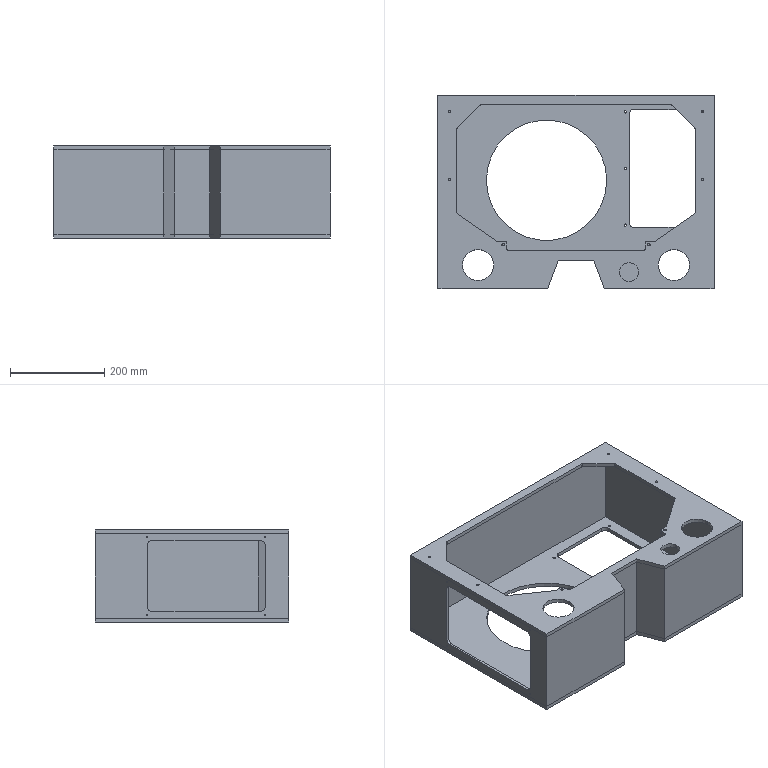Part | STEP file | Tube-changer housing SGN-2-01 | 3 solids | 122 faces | box 585 x 410 x 196 mm | volume 3418245 mm3 | cylinder 64 | plane 58 | commonest cylinder face diameters 5 x24 10 x12 3.3 x8 20 x8 66 x8 40 x2